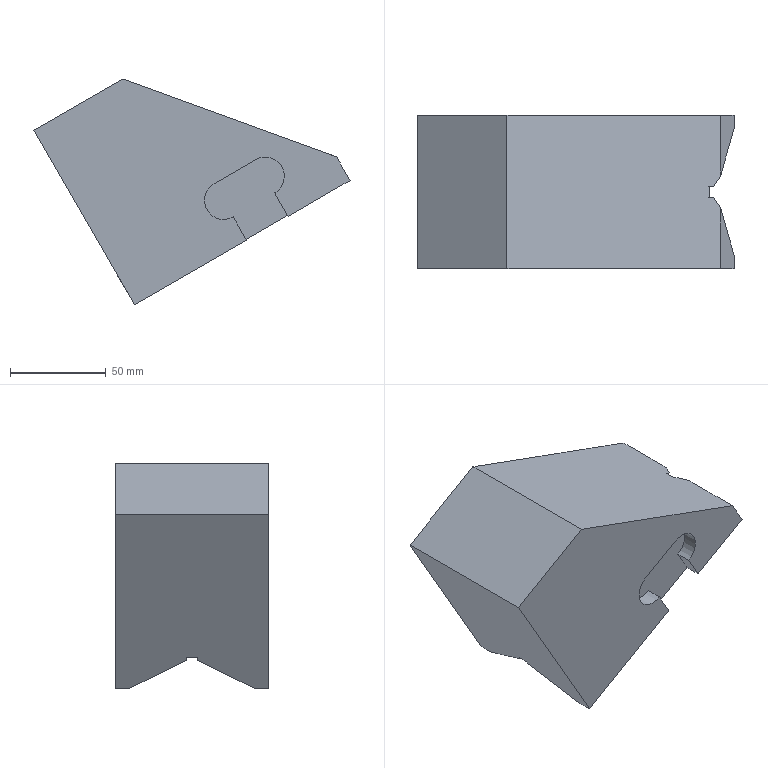Part | NX | features solid 2 | 1 solid | 28 faces | box 164.943 x 80 x 117.764 mm | volume 713626 mm3 | plane 24 | cylinder 4 | commonest cylinder face diameters 20 x4
STEP:
#1=CARTESIAN_POINT('',(760.874,-629.051,126.432));
#2=VERTEX_POINT('',#1);
#3=CARTESIAN_POINT('',(872.234,-629.052,85.9));
#4=VERTEX_POINT('',#3);
#5=CARTESIAN_POINT('',(761.219,-629.051,126.306));
#6=DIRECTION('',(0.9397,-0.000001618,-0.342));
#7=VECTOR('',#6,1000.);
#8=LINE('',#5,#7);
#9=EDGE_CURVE('',#2,#4,#8,.T.);
#10=ORIENTED_EDGE('',*,*,#9,.T.);
#11=CARTESIAN_POINT('',(879.343,-629.052,73.586));
#12=VERTEX_POINT('',#11);
#13=CARTESIAN_POINT('',(853.093,-629.052,119.052));
#14=DIRECTION('',(0.5,-0.000000963,-0.866));
#15=VECTOR('',#14,1000.);
#16=LINE('',#13,#15);
#17=EDGE_CURVE('',#4,#12,#16,.T.);
#18=ORIENTED_EDGE('',*,*,#17,.T.);
#19=CARTESIAN_POINT('',(847.008,-629.052,54.917));
#20=VERTEX_POINT('',#19);
#21=CARTESIAN_POINT('',(823.192,-629.051,41.167));
#22=DIRECTION('',(-0.866,0.00000137,-0.5));
#23=VECTOR('',#22,1000.);
#24=LINE('',#21,#23);
#25=EDGE_CURVE('',#12,#20,#24,.T.);
#26=ORIENTED_EDGE('',*,*,#25,.T.);
#27=CARTESIAN_POINT('',(840.008,-629.051,67.042));
#28=VERTEX_POINT('',#27);
#29=CARTESIAN_POINT('',(840.008,-629.051,67.042));
#30=DIRECTION('',(-0.5,0.000000963,0.866));
#31=VECTOR('',#30,1000.);
#32=LINE('',#29,#31);
#33=EDGE_CURVE('',#20,#28,#32,.T.);
#34=ORIENTED_EDGE('',*,*,#33,.T.);
#35=CARTESIAN_POINT('',(830.008,-629.051,84.362));
#36=VERTEX_POINT('',#35);
#37=CARTESIAN_POINT('',(835.008,-629.051,75.702));
#38=DIRECTION('',(0.000001668,1.,-0.000000149));
#39=DIRECTION('',(-0.9962,0.000001649,-0.08716));
#40=AXIS2_PLACEMENT_3D('',#37,#38,#39);
#41=CIRCLE('',#40,10.);
#42=EDGE_CURVE('',#36,#28,#41,.T.);
#43=ORIENTED_EDGE('',*,*,#42,.F.);
#44=CARTESIAN_POINT('',(808.357,-629.051,71.862));
#45=VERTEX_POINT('',#44);
#46=CARTESIAN_POINT('',(808.357,-629.051,71.862));
#47=DIRECTION('',(0.866,-0.00000137,0.5));
#48=VECTOR('',#47,1000.);
#49=LINE('',#46,#48);
#50=EDGE_CURVE('',#45,#36,#49,.T.);
#51=ORIENTED_EDGE('',*,*,#50,.F.);
#52=CARTESIAN_POINT('',(818.357,-629.051,54.542));
#53=VERTEX_POINT('',#52);
#54=CARTESIAN_POINT('',(813.357,-629.051,63.202));
#55=DIRECTION('',(0.000001668,1.,-0.000000149));
#56=DIRECTION('',(-0.9962,0.000001649,-0.08716));
#57=AXIS2_PLACEMENT_3D('',#54,#55,#56);
#58=CIRCLE('',#57,10.);
#59=EDGE_CURVE('',#53,#45,#58,.T.);
#60=ORIENTED_EDGE('',*,*,#59,.F.);
#61=CARTESIAN_POINT('',(825.357,-629.051,42.417));
#62=VERTEX_POINT('',#61);
#63=CARTESIAN_POINT('',(833.357,-629.051,28.561));
#64=DIRECTION('',(-0.5,0.000000963,0.866));
#65=VECTOR('',#64,1000.);
#66=LINE('',#63,#65);
#67=EDGE_CURVE('',#62,#53,#66,.T.);
#68=ORIENTED_EDGE('',*,*,#67,.F.);
#69=CARTESIAN_POINT('',(766.9,-629.051,8.667));
#70=VERTEX_POINT('',#69);
#71=CARTESIAN_POINT('',(823.192,-629.051,41.167));
#72=DIRECTION('',(-0.866,0.00000137,-0.5));
#73=VECTOR('',#72,1000.);
#74=LINE('',#71,#73);
#75=EDGE_CURVE('',#62,#70,#74,.T.);
#76=ORIENTED_EDGE('',*,*,#75,.T.);
#77=CARTESIAN_POINT('',(714.4,-629.051,99.6));
#78=VERTEX_POINT('',#77);
#79=CARTESIAN_POINT('',(740.65,-629.051,54.134));
#80=DIRECTION('',(-0.5,0.000000963,0.866));
#81=VECTOR('',#80,1000.);
#82=LINE('',#79,#81);
#83=EDGE_CURVE('',#70,#78,#82,.T.);
#84=ORIENTED_EDGE('',*,*,#83,.T.);
#85=CARTESIAN_POINT('',(770.692,-629.051,132.1));
#86=DIRECTION('',(0.866,-0.00000137,0.5));
#87=VECTOR('',#86,1000.);
#88=LINE('',#85,#87);
#89=EDGE_CURVE('',#78,#2,#88,.T.);
#90=ORIENTED_EDGE('',*,*,#89,.T.);
#91=EDGE_LOOP('',(#10,#18,#26,#34,#43,#51,#60,#68,#76,#84,#90));
#92=FACE_BOUND('',#91,.T.);
#93=CARTESIAN_POINT('',(796.942,-629.051,86.634));
#94=DIRECTION('',(0.000001668,1.,-0.000000149));
#95=DIRECTION('',(0.866,-0.00000137,0.5));
#96=AXIS2_PLACEMENT_3D('',#93,#94,#95);
#97=PLANE('',#96);
#98=ADVANCED_FACE('',(#92),#97,.T.);
#99=CARTESIAN_POINT('',(825.357,-636.143,42.417));
#100=VERTEX_POINT('',#99);
#101=CARTESIAN_POINT('',(766.9,-636.142,8.667));
#102=VERTEX_POINT('',#101);
#103=CARTESIAN_POINT('',(879.484,-636.143,73.667));
#104=DIRECTION('',(-0.866,0.00000137,-0.5));
#105=VECTOR('',#104,1000.);
#106=LINE('',#103,#105);
#107=EDGE_CURVE('',#100,#102,#106,.T.);
#108=ORIENTED_EDGE('',*,*,#107,.T.);
#109=CARTESIAN_POINT('',(766.9,-629.051,8.667));
#110=DIRECTION('',(-0.000001668,-1.,0.000000149));
#111=VECTOR('',#110,1000.);
#112=LINE('',#109,#111);
#113=EDGE_CURVE('',#70,#102,#112,.T.);
#114=ORIENTED_EDGE('',*,*,#113,.F.);
#115=ORIENTED_EDGE('',*,*,#75,.F.);
#116=CARTESIAN_POINT('',(825.357,-629.051,42.417));
#117=DIRECTION('',(0.000001668,1.,-0.000000149));
#118=VECTOR('',#117,1000.);
#119=LINE('',#116,#118);
#120=EDGE_CURVE('',#100,#62,#119,.T.);
#121=ORIENTED_EDGE('',*,*,#120,.F.);
#122=EDGE_LOOP('',(#108,#114,#115,#121));
#123=FACE_BOUND('',#122,.T.);
#124=CARTESIAN_POINT('',(823.192,-629.051,41.167));
#125=DIRECTION('',(0.5,-0.000000963,-0.866));
#126=DIRECTION('',(0.000001668,1.,-0.000000149));
#127=AXIS2_PLACEMENT_3D('',#124,#125,#126);
#128=PLANE('',#127);
#129=ADVANCED_FACE('',(#123),#128,.T.);
#130=CARTESIAN_POINT('',(872.233,-660.77,85.9));
#131=VERTEX_POINT('',#130);
#132=CARTESIAN_POINT('',(868.493,-666.052,87.261));
#133=VERTEX_POINT('',#132);
#134=CARTESIAN_POINT('',(869.088,-665.211,87.045));
#135=DIRECTION('',(-0.5656,-0.7986,0.2059));
#136=VECTOR('',#135,1000.);
#137=LINE('',#134,#136);
#138=EDGE_CURVE('',#131,#133,#137,.T.);
#139=ORIENTED_EDGE('',*,*,#138,.T.);
#140=CARTESIAN_POINT('',(758.266,-666.051,23.622));
#141=VERTEX_POINT('',#140);
#142=CARTESIAN_POINT('',(870.849,-666.052,88.622));
#143=DIRECTION('',(-0.866,0.00000137,-0.5));
#144=VECTOR('',#143,1000.);
#145=LINE('',#142,#144);
#146=EDGE_CURVE('',#133,#141,#145,.T.);
#147=ORIENTED_EDGE('',*,*,#146,.T.);
#148=CARTESIAN_POINT('',(758.266,-666.051,23.622));
#149=DIRECTION('',(0.25,0.866,-0.433));
#150=VECTOR('',#149,1000.);
#151=LINE('',#148,#150);
#152=EDGE_CURVE('',#141,#102,#151,.T.);
#153=ORIENTED_EDGE('',*,*,#152,.T.);
#154=ORIENTED_EDGE('',*,*,#107,.F.);
#155=CARTESIAN_POINT('',(825.095,-637.051,42.872));
#156=VERTEX_POINT('',#155);
#157=CARTESIAN_POINT('',(816.723,-666.051,57.372));
#158=DIRECTION('',(0.25,0.866,-0.433));
#159=VECTOR('',#158,1000.);
#160=LINE('',#157,#159);
#161=EDGE_CURVE('',#156,#100,#160,.T.);
#162=ORIENTED_EDGE('',*,*,#161,.F.);
#163=CARTESIAN_POINT('',(846.745,-637.052,55.372));
#164=VERTEX_POINT('',#163);
#165=CARTESIAN_POINT('',(879.221,-637.052,74.122));
#166=DIRECTION('',(-0.866,0.00000137,-0.5));
#167=VECTOR('',#166,1000.);
#168=LINE('',#165,#167);
#169=EDGE_CURVE('',#164,#156,#168,.T.);
#170=ORIENTED_EDGE('',*,*,#169,.F.);
#171=CARTESIAN_POINT('',(847.008,-636.143,54.917));
#172=VERTEX_POINT('',#171);
#173=CARTESIAN_POINT('',(838.374,-666.051,69.872));
#174=DIRECTION('',(0.25,0.866,-0.433));
#175=VECTOR('',#174,1000.);
#176=LINE('',#173,#175);
#177=EDGE_CURVE('',#164,#172,#176,.T.);
#178=ORIENTED_EDGE('',*,*,#177,.T.);
#179=CARTESIAN_POINT('',(879.343,-636.143,73.586));
#180=VERTEX_POINT('',#179);
#181=CARTESIAN_POINT('',(879.484,-636.143,73.667));
#182=DIRECTION('',(-0.866,0.00000137,-0.5));
#183=VECTOR('',#182,1000.);
#184=LINE('',#181,#183);
#185=EDGE_CURVE('',#180,#172,#184,.T.);
#186=ORIENTED_EDGE('',*,*,#185,.F.);
#187=CARTESIAN_POINT('',(870.709,-666.052,88.541));
#188=DIRECTION('',(0.25,0.866,-0.433));
#189=VECTOR('',#188,1000.);
#190=LINE('',#187,#189);
#191=EDGE_CURVE('',#131,#180,#190,.T.);
#192=ORIENTED_EDGE('',*,*,#191,.F.);
#193=EDGE_LOOP('',(#139,#147,#153,#154,#162,#170,#178,#186,#192));
#194=FACE_BOUND('',#193,.T.);
#195=CARTESIAN_POINT('',(870.849,-666.052,88.622));
#196=DIRECTION('',(0.433,-0.5,-0.75));
#197=DIRECTION('',(0.25,0.866,-0.433));
#198=AXIS2_PLACEMENT_3D('',#195,#196,#197);
#199=PLANE('',#198);
#200=ADVANCED_FACE('',(#194),#199,.T.);
#201=CARTESIAN_POINT('',(879.343,-701.961,73.586));
#202=VERTEX_POINT('',#201);
#203=CARTESIAN_POINT('',(847.007,-701.96,54.917));
#204=VERTEX_POINT('',#203);
#205=CARTESIAN_POINT('',(879.483,-701.961,73.667));
#206=DIRECTION('',(-0.866,0.00000137,-0.5));
#207=VECTOR('',#206,1000.);
#208=LINE('',#205,#207);
#209=EDGE_CURVE('',#202,#204,#208,.T.);
#210=ORIENTED_EDGE('',*,*,#209,.F.);
#211=CARTESIAN_POINT('',(879.343,-709.052,73.586));
#212=VERTEX_POINT('',#211);
#213=CARTESIAN_POINT('',(879.343,-629.052,73.586));
#214=DIRECTION('',(-0.000001668,-1.,0.000000149));
#215=VECTOR('',#214,1000.);
#216=LINE('',#213,#215);
#217=EDGE_CURVE('',#202,#212,#216,.T.);
#218=ORIENTED_EDGE('',*,*,#217,.T.);
#219=CARTESIAN_POINT('',(847.007,-709.052,54.917));
#220=VERTEX_POINT('',#219);
#221=CARTESIAN_POINT('',(823.192,-709.051,41.167));
#222=DIRECTION('',(0.866,-0.00000137,0.5));
#223=VECTOR('',#222,1000.);
#224=LINE('',#221,#223);
#225=EDGE_CURVE('',#220,#212,#224,.T.);
#226=ORIENTED_EDGE('',*,*,#225,.F.);
#227=CARTESIAN_POINT('',(847.008,-629.052,54.917));
#228=DIRECTION('',(-0.000001668,-1.,0.000000149));
#229=VECTOR('',#228,1000.);
#230=LINE('',#227,#229);
#231=EDGE_CURVE('',#204,#220,#230,.T.);
#232=ORIENTED_EDGE('',*,*,#231,.F.);
#233=EDGE_LOOP('',(#210,#218,#226,#232));
#234=FACE_BOUND('',#233,.T.);
#235=CARTESIAN_POINT('',(823.192,-629.051,41.167));
#236=DIRECTION('',(0.5,-0.000000963,-0.866));
#237=DIRECTION('',(0.000001668,1.,-0.000000149));
#238=AXIS2_PLACEMENT_3D('',#235,#236,#237);
#239=PLANE('',#238);
#240=ADVANCED_FACE('',(#234),#239,.T.);
#241=CARTESIAN_POINT('',(847.008,-629.052,54.917));
#242=DIRECTION('',(0.000001668,1.,-0.000000149));
#243=VECTOR('',#242,1000.);
#244=LINE('',#241,#243);
#245=EDGE_CURVE('',#172,#20,#244,.T.);
#246=ORIENTED_EDGE('',*,*,#245,.T.);
#247=ORIENTED_EDGE('',*,*,#25,.F.);
#248=CARTESIAN_POINT('',(879.343,-629.052,73.586));
#249=DIRECTION('',(-0.000001668,-1.,0.000000149));
#250=VECTOR('',#249,1000.);
#251=LINE('',#248,#250);
#252=EDGE_CURVE('',#12,#180,#251,.T.);
#253=ORIENTED_EDGE('',*,*,#252,.T.);
#254=ORIENTED_EDGE('',*,*,#185,.T.);
#255=EDGE_LOOP('',(#246,#247,#253,#254));
#256=FACE_BOUND('',#255,.T.);
#257=CARTESIAN_POINT('',(823.192,-629.051,41.167));
#258=DIRECTION('',(0.5,-0.000000963,-0.866));
#259=DIRECTION('',(0.000001668,1.,-0.000000149));
#260=AXIS2_PLACEMENT_3D('',#257,#258,#259);
#261=PLANE('',#260);
#262=ADVANCED_FACE('',(#256),#261,.T.);
#263=CARTESIAN_POINT('',(825.357,-701.96,42.417));
#264=VERTEX_POINT('',#263);
#265=CARTESIAN_POINT('',(825.357,-709.051,42.417));
#266=VERTEX_POINT('',#265);
#267=CARTESIAN_POINT('',(825.357,-629.051,42.417));
#268=DIRECTION('',(-0.000001668,-1.,0.000000149));
#269=VECTOR('',#268,1000.);
#270=LINE('',#267,#269);
#271=EDGE_CURVE('',#264,#266,#270,.T.);
#272=ORIENTED_EDGE('',*,*,#271,.T.);
#273=CARTESIAN_POINT('',(766.9,-709.051,8.667));
#274=VERTEX_POINT('',#273);
#275=CARTESIAN_POINT('',(823.192,-709.051,41.167));
#276=DIRECTION('',(0.866,-0.00000137,0.5));
#277=VECTOR('',#276,1000.);
#278=LINE('',#275,#277);
#279=EDGE_CURVE('',#274,#266,#278,.T.);
#280=ORIENTED_EDGE('',*,*,#279,.F.);
#281=CARTESIAN_POINT('',(766.9,-701.96,8.667));
#282=VERTEX_POINT('',#281);
#283=CARTESIAN_POINT('',(766.9,-629.051,8.667));
#284=DIRECTION('',(-0.000001668,-1.,0.000000149));
#285=VECTOR('',#284,1000.);
#286=LINE('',#283,#285);
#287=EDGE_CURVE('',#282,#274,#286,.T.);
#288=ORIENTED_EDGE('',*,*,#287,.F.);
#289=CARTESIAN_POINT('',(879.483,-701.961,73.667));
#290=DIRECTION('',(-0.866,0.00000137,-0.5));
#291=VECTOR('',#290,1000.);
#292=LINE('',#289,#291);
#293=EDGE_CURVE('',#264,#282,#292,.T.);
#294=ORIENTED_EDGE('',*,*,#293,.F.);
#295=EDGE_LOOP('',(#272,#280,#288,#294));
#296=FACE_BOUND('',#295,.T.);
#297=CARTESIAN_POINT('',(823.192,-629.051,41.167));
#298=DIRECTION('',(0.5,-0.000000963,-0.866));
#299=DIRECTION('',(0.000001668,1.,-0.000000149));
#300=AXIS2_PLACEMENT_3D('',#297,#298,#299);
#301=PLANE('',#300);
#302=ADVANCED_FACE('',(#296),#301,.T.);
#303=CARTESIAN_POINT('',(872.233,-709.052,85.9));
#304=DIRECTION('',(0.000001668,1.,-0.000000149));
#305=VECTOR('',#304,1000.);
#306=LINE('',#303,#305);
#307=EDGE_CURVE('',#131,#4,#306,.T.);
#308=ORIENTED_EDGE('',*,*,#307,.F.);
#309=ORIENTED_EDGE('',*,*,#191,.T.);
#310=ORIENTED_EDGE('',*,*,#252,.F.);
#311=ORIENTED_EDGE('',*,*,#17,.F.);
#312=EDGE_LOOP('',(#308,#309,#310,#311));
#313=FACE_BOUND('',#312,.T.);
#314=CARTESIAN_POINT('',(853.093,-629.052,119.052));
#315=DIRECTION('',(0.866,-0.00000137,0.5));
#316=DIRECTION('',(-0.000001668,-1.,0.000000149));
#317=AXIS2_PLACEMENT_3D('',#314,#315,#316);
#318=PLANE('',#317);
#319=ADVANCED_FACE('',(#313),#318,.T.);
#320=CARTESIAN_POINT('',(872.233,-709.052,85.9));
#321=VERTEX_POINT('',#320);
#322=CARTESIAN_POINT('',(872.233,-677.333,85.9));
#323=VERTEX_POINT('',#322);
#324=CARTESIAN_POINT('',(872.233,-709.052,85.9));
#325=DIRECTION('',(0.000001668,1.,-0.000000149));
#326=VECTOR('',#325,1000.);
#327=LINE('',#324,#326);
#328=EDGE_CURVE('',#321,#323,#327,.T.);
#329=ORIENTED_EDGE('',*,*,#328,.F.);
#330=CARTESIAN_POINT('',(853.093,-709.052,119.052));
#331=DIRECTION('',(-0.5,0.000000963,0.866));
#332=VECTOR('',#331,1000.);
#333=LINE('',#330,#332);
#334=EDGE_CURVE('',#212,#321,#333,.T.);
#335=ORIENTED_EDGE('',*,*,#334,.F.);
#336=ORIENTED_EDGE('',*,*,#217,.F.);
#337=CARTESIAN_POINT('',(879.343,-701.961,73.586));
#338=DIRECTION('',(-0.25,0.866,0.433));
#339=VECTOR('',#338,1000.);
#340=LINE('',#337,#339);
#341=EDGE_CURVE('',#202,#323,#340,.T.);
#342=ORIENTED_EDGE('',*,*,#341,.T.);
#343=EDGE_LOOP('',(#329,#335,#336,#342));
#344=FACE_BOUND('',#343,.T.);
#345=CARTESIAN_POINT('',(853.093,-629.052,119.052));
#346=DIRECTION('',(0.866,-0.00000137,0.5));
#347=DIRECTION('',(-0.000001668,-1.,0.000000149));
#348=AXIS2_PLACEMENT_3D('',#345,#346,#347);
#349=PLANE('',#348);
#350=ADVANCED_FACE('',(#344),#349,.T.);
#351=CARTESIAN_POINT('',(757.4,-666.051,25.122));
#352=VERTEX_POINT('',#351);
#353=CARTESIAN_POINT('',(757.4,-666.051,25.122));
#354=DIRECTION('',(0.5,-0.000000963,-0.866));
#355=VECTOR('',#354,1000.);
#356=LINE('',#353,#355);
#357=EDGE_CURVE('',#352,#141,#356,.T.);
#358=ORIENTED_EDGE('',*,*,#357,.F.);
#359=CARTESIAN_POINT('',(757.4,-672.051,25.122));
#360=VERTEX_POINT('',#359);
#361=CARTESIAN_POINT('',(757.4,-672.051,25.122));
#362=DIRECTION('',(0.000001668,1.,-0.000000149));
#363=VECTOR('',#362,1000.);
#364=LINE('',#361,#363);
#365=EDGE_CURVE('',#360,#352,#364,.T.);
#366=ORIENTED_EDGE('',*,*,#365,.F.);
#367=CARTESIAN_POINT('',(758.266,-672.051,23.622));
#368=VERTEX_POINT('',#367);
#369=CARTESIAN_POINT('',(758.266,-672.051,23.622));
#370=DIRECTION('',(-0.5,0.000000963,0.866));
#371=VECTOR('',#370,1000.);
#372=LINE('',#369,#371);
#373=EDGE_CURVE('',#368,#360,#372,.T.);
#374=ORIENTED_EDGE('',*,*,#373,.F.);
#375=CARTESIAN_POINT('',(766.9,-701.96,8.667));
#376=DIRECTION('',(-0.25,0.866,0.433));
#377=VECTOR('',#376,1000.);
#378=LINE('',#375,#377);
#379=EDGE_CURVE('',#282,#368,#378,.T.);
#380=ORIENTED_EDGE('',*,*,#379,.F.);
#381=ORIENTED_EDGE('',*,*,#287,.T.);
#382=CARTESIAN_POINT('',(714.4,-709.051,99.6));
#383=VERTEX_POINT('',#382);
#384=CARTESIAN_POINT('',(740.65,-709.051,54.134));
#385=DIRECTION('',(0.5,-0.000000963,-0.866));
#386=VECTOR('',#385,1000.);
#387=LINE('',#384,#386);
#388=EDGE_CURVE('',#383,#274,#387,.T.);
#389=ORIENTED_EDGE('',*,*,#388,.F.);
#390=CARTESIAN_POINT('',(714.4,-629.051,99.6));
#391=DIRECTION('',(-0.000001668,-1.,0.000000149));
#392=VECTOR('',#391,1000.);
#393=LINE('',#390,#392);
#394=EDGE_CURVE('',#78,#383,#393,.T.);
#395=ORIENTED_EDGE('',*,*,#394,.F.);
#396=ORIENTED_EDGE('',*,*,#83,.F.);
#397=ORIENTED_EDGE('',*,*,#113,.T.);
#398=ORIENTED_EDGE('',*,*,#152,.F.);
#399=EDGE_LOOP('',(#358,#366,#374,#380,#381,#389,#395,#396,#397,#398));
#400=FACE_BOUND('',#399,.T.);
#401=CARTESIAN_POINT('',(740.65,-629.051,54.134));
#402=DIRECTION('',(-0.866,0.00000137,-0.5));
#403=DIRECTION('',(0.000001668,1.,-0.000000149));
#404=AXIS2_PLACEMENT_3D('',#401,#402,#403);
#405=PLANE('',#404);
#406=ADVANCED_FACE('',(#400),#405,.T.);
#407=CARTESIAN_POINT('',(760.874,-709.051,126.432));
#408=VERTEX_POINT('',#407);
#409=CARTESIAN_POINT('',(761.219,-709.051,126.306));
#410=DIRECTION('',(0.9397,-0.000001618,-0.342));
#411=VECTOR('',#410,1000.);
#412=LINE('',#409,#411);
#413=EDGE_CURVE('',#408,#321,#412,.T.);
#414=ORIENTED_EDGE('',*,*,#413,.F.);
#415=CARTESIAN_POINT('',(770.692,-709.051,132.1));
#416=DIRECTION('',(-0.866,0.00000137,-0.5));
#417=VECTOR('',#416,1000.);
#418=LINE('',#415,#417);
#419=EDGE_CURVE('',#408,#383,#418,.T.);
#420=ORIENTED_EDGE('',*,*,#419,.T.);
#421=ORIENTED_EDGE('',*,*,#388,.T.);
#422=ORIENTED_EDGE('',*,*,#279,.T.);
#423=CARTESIAN_POINT('',(818.357,-709.051,54.542));
#424=VERTEX_POINT('',#423);
#425=CARTESIAN_POINT('',(833.357,-709.051,28.561));
#426=DIRECTION('',(-0.5,0.000000963,0.866));
#427=VECTOR('',#426,1000.);
#428=LINE('',#425,#427);
#429=EDGE_CURVE('',#266,#424,#428,.T.);
#430=ORIENTED_EDGE('',*,*,#429,.T.);
#431=CARTESIAN_POINT('',(808.357,-709.051,71.862));
#432=VERTEX_POINT('',#431);
#433=CARTESIAN_POINT('',(813.357,-709.051,63.202));
#434=DIRECTION('',(0.000001668,1.,-0.000000149));
#435=DIRECTION('',(-0.9962,0.000001649,-0.08716));
#436=AXIS2_PLACEMENT_3D('',#433,#434,#435);
#437=CIRCLE('',#436,10.);
#438=EDGE_CURVE('',#424,#432,#437,.T.);
#439=ORIENTED_EDGE('',*,*,#438,.T.);
#440=CARTESIAN_POINT('',(830.007,-709.051,84.362));
#441=VERTEX_POINT('',#440);
#442=CARTESIAN_POINT('',(830.007,-709.051,84.362));
#443=DIRECTION('',(-0.866,0.00000137,-0.5));
#444=VECTOR('',#443,1000.);
#445=LINE('',#442,#444);
#446=EDGE_CURVE('',#441,#432,#445,.T.);
#447=ORIENTED_EDGE('',*,*,#446,.F.);
#448=CARTESIAN_POINT('',(840.007,-709.051,67.042));
#449=VERTEX_POINT('',#448);
#450=CARTESIAN_POINT('',(835.007,-709.051,75.702));
#451=DIRECTION('',(0.000001668,1.,-0.000000149));
#452=DIRECTION('',(-0.9962,0.000001649,-0.08716));
#453=AXIS2_PLACEMENT_3D('',#450,#451,#452);
#454=CIRCLE('',#453,10.);
#455=EDGE_CURVE('',#441,#449,#454,.T.);
#456=ORIENTED_EDGE('',*,*,#455,.T.);
#457=CARTESIAN_POINT('',(855.007,-709.052,41.061));
#458=DIRECTION('',(-0.5,0.000000963,0.866));
#459=VECTOR('',#458,1000.);
#460=LINE('',#457,#459);
#461=EDGE_CURVE('',#220,#449,#460,.T.);
#462=ORIENTED_EDGE('',*,*,#461,.F.);
#463=ORIENTED_EDGE('',*,*,#225,.T.);
#464=ORIENTED_EDGE('',*,*,#334,.T.);
#465=EDGE_LOOP('',(#414,#420,#421,#422,#430,#439,#447,#456,#462,#463,#464));
#466=FACE_BOUND('',#465,.T.);
#467=CARTESIAN_POINT('',(796.942,-709.051,86.634));
#468=DIRECTION('',(-0.000001668,-1.,0.000000149));
#469=DIRECTION('',(-0.866,0.00000137,-0.5));
#470=AXIS2_PLACEMENT_3D('',#467,#468,#469);
#471=PLANE('',#470);
#472=ADVANCED_FACE('',(#466),#471,.T.);
#473=CARTESIAN_POINT('',(760.874,-629.051,126.432));
#474=DIRECTION('',(0.000001668,1.,-0.000000149));
#475=VECTOR('',#474,1000.);
#476=LINE('',#473,#475);
#477=EDGE_CURVE('',#408,#2,#476,.T.);
#478=ORIENTED_EDGE('',*,*,#477,.T.);
#479=ORIENTED_EDGE('',*,*,#89,.F.);
#480=ORIENTED_EDGE('',*,*,#394,.T.);
#481=ORIENTED_EDGE('',*,*,#419,.F.);
#482=EDGE_LOOP('',(#478,#479,#480,#481));
#483=FACE_BOUND('',#482,.T.);
#484=CARTESIAN_POINT('',(770.692,-629.051,132.1));
#485=DIRECTION('',(-0.5,0.000000963,0.866));
#486=DIRECTION('',(-0.000001668,-1.,0.000000149));
#487=AXIS2_PLACEMENT_3D('',#484,#485,#486);
#488=PLANE('',#487);
#489=ADVANCED_FACE('',(#483),#488,.T.);
#490=CARTESIAN_POINT('',(866.368,-672.052,88.035));
#491=VERTEX_POINT('',#490);
#492=CARTESIAN_POINT('',(868.493,-672.052,87.261));
#493=VERTEX_POINT('',#492);
#494=CARTESIAN_POINT('',(870.137,-672.052,86.663));
#495=DIRECTION('',(0.9397,-0.000001618,-0.342));
#496=VECTOR('',#495,1000.);
#497=LINE('',#494,#496);
#498=EDGE_CURVE('',#491,#493,#497,.T.);
#499=ORIENTED_EDGE('',*,*,#498,.T.);
#500=CARTESIAN_POINT('',(870.849,-672.052,88.622));
#501=DIRECTION('',(-0.866,0.00000137,-0.5));
#502=VECTOR('',#501,1000.);
#503=LINE('',#500,#502);
#504=EDGE_CURVE('',#493,#368,#503,.T.);
#505=ORIENTED_EDGE('',*,*,#504,.T.);
#506=ORIENTED_EDGE('',*,*,#373,.T.);
#507=CARTESIAN_POINT('',(869.983,-672.052,90.122));
#508=DIRECTION('',(-0.866,0.00000137,-0.5));
#509=VECTOR('',#508,1000.);
#510=LINE('',#507,#509);
#511=EDGE_CURVE('',#491,#360,#510,.T.);
#512=ORIENTED_EDGE('',*,*,#511,.F.);
#513=EDGE_LOOP('',(#499,#505,#506,#512));
#514=FACE_BOUND('',#513,.T.);
#515=CARTESIAN_POINT('',(870.849,-672.052,88.622));
#516=DIRECTION('',(0.000001668,1.,-0.000000149));
#517=DIRECTION('',(-0.5,0.000000963,0.866));
#518=AXIS2_PLACEMENT_3D('',#515,#516,#517);
#519=PLANE('',#518);
#520=ADVANCED_FACE('',(#514),#519,.T.);
#521=CARTESIAN_POINT('',(866.368,-666.052,88.035));
#522=VERTEX_POINT('',#521);
#523=CARTESIAN_POINT('',(866.368,-672.052,88.035));
#524=DIRECTION('',(-0.000001668,-1.,0.000000149));
#525=VECTOR('',#524,1000.);
#526=LINE('',#523,#525);
#527=EDGE_CURVE('',#522,#491,#526,.T.);
#528=ORIENTED_EDGE('',*,*,#527,.T.);
#529=ORIENTED_EDGE('',*,*,#511,.T.);
#530=ORIENTED_EDGE('',*,*,#365,.T.);
#531=CARTESIAN_POINT('',(869.983,-666.052,90.122));
#532=DIRECTION('',(-0.866,0.00000137,-0.5));
#533=VECTOR('',#532,1000.);
#534=LINE('',#531,#533);
#535=EDGE_CURVE('',#522,#352,#534,.T.);
#536=ORIENTED_EDGE('',*,*,#535,.F.);
#537=EDGE_LOOP('',(#528,#529,#530,#536));
#538=FACE_BOUND('',#537,.T.);
#539=CARTESIAN_POINT('',(869.983,-672.052,90.122));
#540=DIRECTION('',(0.5,-0.000000963,-0.866));
#541=DIRECTION('',(0.000001668,1.,-0.000000149));
#542=AXIS2_PLACEMENT_3D('',#539,#540,#541);
#543=PLANE('',#542);
#544=ADVANCED_FACE('',(#538),#543,.T.);
#545=CARTESIAN_POINT('',(868.89,-666.052,87.117));
#546=DIRECTION('',(-0.9397,0.000001618,0.342));
#547=VECTOR('',#546,1000.);
#548=LINE('',#545,#547);
#549=EDGE_CURVE('',#133,#522,#548,.T.);
#550=ORIENTED_EDGE('',*,*,#549,.T.);
#551=ORIENTED_EDGE('',*,*,#535,.T.);
#552=ORIENTED_EDGE('',*,*,#357,.T.);
#553=ORIENTED_EDGE('',*,*,#146,.F.);
#554=EDGE_LOOP('',(#550,#551,#552,#553));
#555=FACE_BOUND('',#554,.T.);
#556=CARTESIAN_POINT('',(869.983,-666.052,90.122));
#557=DIRECTION('',(-0.000001668,-1.,0.000000149));
#558=DIRECTION('',(0.5,-0.000000963,-0.866));
#559=AXIS2_PLACEMENT_3D('',#556,#557,#558);
#560=PLANE('',#559);
#561=ADVANCED_FACE('',(#555),#560,.T.);
#562=CARTESIAN_POINT('',(887.1,-698.325,80.489));
#563=DIRECTION('',(0.5656,-0.7986,-0.2059));
#564=VECTOR('',#563,1000.);
#565=LINE('',#562,#564);
#566=EDGE_CURVE('',#493,#323,#565,.T.);
#567=ORIENTED_EDGE('',*,*,#566,.T.);
#568=ORIENTED_EDGE('',*,*,#341,.F.);
#569=ORIENTED_EDGE('',*,*,#209,.T.);
#570=CARTESIAN_POINT('',(846.745,-701.052,55.372));
#571=VERTEX_POINT('',#570);
#572=CARTESIAN_POINT('',(847.007,-701.96,54.917));
#573=DIRECTION('',(0.25,-0.866,-0.433));
#574=VECTOR('',#573,1000.);
#575=LINE('',#572,#574);
#576=EDGE_CURVE('',#571,#204,#575,.T.);
#577=ORIENTED_EDGE('',*,*,#576,.F.);
#578=CARTESIAN_POINT('',(825.094,-701.051,42.872));
#579=VERTEX_POINT('',#578);
#580=CARTESIAN_POINT('',(879.221,-701.052,74.122));
#581=DIRECTION('',(0.866,-0.00000137,0.5));
#582=VECTOR('',#581,1000.);
#583=LINE('',#580,#582);
#584=EDGE_CURVE('',#579,#571,#583,.T.);
#585=ORIENTED_EDGE('',*,*,#584,.F.);
#586=CARTESIAN_POINT('',(825.357,-701.96,42.417));
#587=DIRECTION('',(0.25,-0.866,-0.433));
#588=VECTOR('',#587,1000.);
#589=LINE('',#586,#588);
#590=EDGE_CURVE('',#579,#264,#589,.T.);
#591=ORIENTED_EDGE('',*,*,#590,.T.);
#592=ORIENTED_EDGE('',*,*,#293,.T.);
#593=ORIENTED_EDGE('',*,*,#379,.T.);
#594=ORIENTED_EDGE('',*,*,#504,.F.);
#595=EDGE_LOOP('',(#567,#568,#569,#577,#585,#591,#592,#593,#594));
#596=FACE_BOUND('',#595,.T.);
#597=CARTESIAN_POINT('',(879.483,-701.961,73.667));
#598=DIRECTION('',(0.433,0.5,-0.75));
#599=DIRECTION('',(-0.25,0.866,0.433));
#600=AXIS2_PLACEMENT_3D('',#597,#598,#599);
#601=PLANE('',#600);
#602=ADVANCED_FACE('',(#596),#601,.T.);
#603=ORIENTED_EDGE('',*,*,#438,.F.);
#604=CARTESIAN_POINT('',(818.357,-701.051,54.542));
#605=VERTEX_POINT('',#604);
#606=CARTESIAN_POINT('',(818.357,-701.051,54.542));
#607=DIRECTION('',(-0.000001668,-1.,0.000000149));
#608=VECTOR('',#607,1000.);
#609=LINE('',#606,#608);
#610=EDGE_CURVE('',#605,#424,#609,.T.);
#611=ORIENTED_EDGE('',*,*,#610,.F.);
#612=CARTESIAN_POINT('',(808.357,-701.051,71.862));
#613=VERTEX_POINT('',#612);
#614=CARTESIAN_POINT('',(813.357,-701.051,63.202));
#615=DIRECTION('',(0.000001668,1.,-0.000000149));
#616=DIRECTION('',(-0.9962,0.000001649,-0.08716));
#617=AXIS2_PLACEMENT_3D('',#614,#615,#616);
#618=CIRCLE('',#617,10.);
#619=EDGE_CURVE('',#605,#613,#618,.T.);
#620=ORIENTED_EDGE('',*,*,#619,.T.);
#621=CARTESIAN_POINT('',(808.357,-701.051,71.862));
#622=DIRECTION('',(-0.000001668,-1.,0.000000149));
#623=VECTOR('',#622,1000.);
#624=LINE('',#621,#623);
#625=EDGE_CURVE('',#613,#432,#624,.T.);
#626=ORIENTED_EDGE('',*,*,#625,.T.);
#627=EDGE_LOOP('',(#603,#611,#620,#626));
#628=FACE_BOUND('',#627,.T.);
#629=CARTESIAN_POINT('',(813.357,-701.051,63.202));
#630=DIRECTION('',(-0.000001668,-1.,0.000000149));
#631=DIRECTION('',(-1.,0.000001668,0.000000502));
#632=AXIS2_PLACEMENT_3D('',#629,#630,#631);
#633=CYLINDRICAL_SURFACE('',#632,10.);
#634=ADVANCED_FACE('',(#628),#633,.F.);
#635=ORIENTED_EDGE('',*,*,#446,.T.);
#636=ORIENTED_EDGE('',*,*,#625,.F.);
#637=CARTESIAN_POINT('',(830.007,-701.051,84.362));
#638=VERTEX_POINT('',#637);
#639=CARTESIAN_POINT('',(830.007,-701.051,84.362));
#640=DIRECTION('',(-0.866,0.00000137,-0.5));
#641=VECTOR('',#640,1000.);
#642=LINE('',#639,#641);
#643=EDGE_CURVE('',#638,#613,#642,.T.);
#644=ORIENTED_EDGE('',*,*,#643,.F.);
#645=CARTESIAN_POINT('',(830.007,-701.051,84.362));
#646=DIRECTION('',(-0.000001668,-1.,0.000000149));
#647=VECTOR('',#646,1000.);
#648=LINE('',#645,#647);
#649=EDGE_CURVE('',#638,#441,#648,.T.);
#650=ORIENTED_EDGE('',*,*,#649,.T.);
#651=EDGE_LOOP('',(#635,#636,#644,#650));
#652=FACE_BOUND('',#651,.T.);
#653=CARTESIAN_POINT('',(830.007,-701.051,84.362));
#654=DIRECTION('',(0.5,-0.000000963,-0.866));
#655=DIRECTION('',(-0.866,0.00000137,-0.5));
#656=AXIS2_PLACEMENT_3D('',#653,#654,#655);
#657=PLANE('',#656);
#658=ADVANCED_FACE('',(#652),#657,.T.);
#659=ORIENTED_EDGE('',*,*,#455,.F.);
#660=ORIENTED_EDGE('',*,*,#649,.F.);
#661=CARTESIAN_POINT('',(840.007,-701.051,67.042));
#662=VERTEX_POINT('',#661);
#663=CARTESIAN_POINT('',(835.007,-701.051,75.702));
#664=DIRECTION('',(0.000001668,1.,-0.000000149));
#665=DIRECTION('',(-0.9962,0.000001649,-0.08716));
#666=AXIS2_PLACEMENT_3D('',#663,#664,#665);
#667=CIRCLE('',#666,10.);
#668=EDGE_CURVE('',#638,#662,#667,.T.);
#669=ORIENTED_EDGE('',*,*,#668,.T.);
#670=CARTESIAN_POINT('',(840.007,-701.051,67.042));
#671=DIRECTION('',(-0.000001668,-1.,0.000000149));
#672=VECTOR('',#671,1000.);
#673=LINE('',#670,#672);
#674=EDGE_CURVE('',#662,#449,#673,.T.);
#675=ORIENTED_EDGE('',*,*,#674,.T.);
#676=EDGE_LOOP('',(#659,#660,#669,#675));
#677=FACE_BOUND('',#676,.T.);
#678=CARTESIAN_POINT('',(835.007,-701.051,75.702));
#679=DIRECTION('',(-0.000001668,-1.,0.000000149));
#680=DIRECTION('',(-1.,0.000001668,0.000000502));
#681=AXIS2_PLACEMENT_3D('',#678,#679,#680);
#682=CYLINDRICAL_SURFACE('',#681,10.);
#683=ADVANCED_FACE('',(#677),#682,.F.);
#684=ORIENTED_EDGE('',*,*,#668,.F.);
#685=ORIENTED_EDGE('',*,*,#643,.T.);
#686=ORIENTED_EDGE('',*,*,#619,.F.);
#687=CARTESIAN_POINT('',(833.357,-701.051,28.561));
#688=DIRECTION('',(-0.5,0.000000963,0.866));
#689=VECTOR('',#688,1000.);
#690=LINE('',#687,#689);
#691=EDGE_CURVE('',#579,#605,#690,.T.);
#692=ORIENTED_EDGE('',*,*,#691,.F.);
#693=ORIENTED_EDGE('',*,*,#584,.T.);
#694=CARTESIAN_POINT('',(855.007,-701.052,41.061));
#695=DIRECTION('',(-0.5,0.000000963,0.866));
#696=VECTOR('',#695,1000.);
#697=LINE('',#694,#696);
#698=EDGE_CURVE('',#571,#662,#697,.T.);
#699=ORIENTED_EDGE('',*,*,#698,.T.);
#700=EDGE_LOOP('',(#684,#685,#686,#692,#693,#699));
#701=FACE_BOUND('',#700,.T.);
#702=CARTESIAN_POINT('',(813.357,-701.051,63.202));
#703=DIRECTION('',(-0.000001668,-1.,0.000000149));
#704=DIRECTION('',(-1.,0.000001668,0.000000502));
#705=AXIS2_PLACEMENT_3D('',#702,#703,#704);
#706=PLANE('',#705);
#707=ADVANCED_FACE('',(#701),#706,.T.);
#708=ORIENTED_EDGE('',*,*,#271,.F.);
#709=ORIENTED_EDGE('',*,*,#590,.F.);
#710=ORIENTED_EDGE('',*,*,#691,.T.);
#711=ORIENTED_EDGE('',*,*,#610,.T.);
#712=ORIENTED_EDGE('',*,*,#429,.F.);
#713=EDGE_LOOP('',(#708,#709,#710,#711,#712));
#714=FACE_BOUND('',#713,.T.);
#715=CARTESIAN_POINT('',(833.357,-701.051,28.561));
#716=DIRECTION('',(-0.866,0.00000137,-0.5));
#717=DIRECTION('',(-0.5,0.000000963,0.866));
#718=AXIS2_PLACEMENT_3D('',#715,#716,#717);
#719=PLANE('',#718);
#720=ADVANCED_FACE('',(#714),#719,.F.);
#721=ORIENTED_EDGE('',*,*,#576,.T.);
#722=ORIENTED_EDGE('',*,*,#231,.T.);
#723=ORIENTED_EDGE('',*,*,#461,.T.);
#724=ORIENTED_EDGE('',*,*,#674,.F.);
#725=ORIENTED_EDGE('',*,*,#698,.F.);
#726=EDGE_LOOP('',(#721,#722,#723,#724,#725));
#727=FACE_BOUND('',#726,.T.);
#728=CARTESIAN_POINT('',(855.007,-701.052,41.061));
#729=DIRECTION('',(-0.866,0.00000137,-0.5));
#730=DIRECTION('',(-0.5,0.000000963,0.866));
#731=AXIS2_PLACEMENT_3D('',#728,#729,#730);
#732=PLANE('',#731);
#733=ADVANCED_FACE('',(#727),#732,.T.);
#734=ORIENTED_EDGE('',*,*,#50,.T.);
#735=CARTESIAN_POINT('',(830.008,-637.051,84.362));
#736=VERTEX_POINT('',#735);
#737=CARTESIAN_POINT('',(830.008,-629.051,84.362));
#738=DIRECTION('',(-0.000001668,-1.,0.000000149));
#739=VECTOR('',#738,1000.);
#740=LINE('',#737,#739);
#741=EDGE_CURVE('',#36,#736,#740,.T.);
#742=ORIENTED_EDGE('',*,*,#741,.T.);
#743=CARTESIAN_POINT('',(808.357,-637.051,71.862));
#744=VERTEX_POINT('',#743);
#745=CARTESIAN_POINT('',(808.357,-637.051,71.862));
#746=DIRECTION('',(0.866,-0.00000137,0.5));
#747=VECTOR('',#746,1000.);
#748=LINE('',#745,#747);
#749=EDGE_CURVE('',#744,#736,#748,.T.);
#750=ORIENTED_EDGE('',*,*,#749,.F.);
#751=CARTESIAN_POINT('',(808.357,-637.051,71.862));
#752=DIRECTION('',(0.000001668,1.,-0.000000149));
#753=VECTOR('',#752,1000.);
#754=LINE('',#751,#753);
#755=EDGE_CURVE('',#744,#45,#754,.T.);
#756=ORIENTED_EDGE('',*,*,#755,.T.);
#757=EDGE_LOOP('',(#734,#742,#750,#756));
#758=FACE_BOUND('',#757,.T.);
#759=CARTESIAN_POINT('',(808.357,-637.051,71.862));
#760=DIRECTION('',(0.5,-0.000000963,-0.866));
#761=DIRECTION('',(-0.866,0.00000137,-0.5));
#762=AXIS2_PLACEMENT_3D('',#759,#760,#761);
#763=PLANE('',#762);
#764=ADVANCED_FACE('',(#758),#763,.T.);
#765=CARTESIAN_POINT('',(818.357,-637.051,54.542));
#766=VERTEX_POINT('',#765);
#767=CARTESIAN_POINT('',(818.357,-629.051,54.542));
#768=DIRECTION('',(-0.000001668,-1.,0.000000149));
#769=VECTOR('',#768,1000.);
#770=LINE('',#767,#769);
#771=EDGE_CURVE('',#53,#766,#770,.T.);
#772=ORIENTED_EDGE('',*,*,#771,.T.);
#773=CARTESIAN_POINT('',(833.357,-637.051,28.561));
#774=DIRECTION('',(-0.5,0.000000963,0.866));
#775=VECTOR('',#774,1000.);
#776=LINE('',#773,#775);
#777=EDGE_CURVE('',#156,#766,#776,.T.);
#778=ORIENTED_EDGE('',*,*,#777,.F.);
#779=ORIENTED_EDGE('',*,*,#161,.T.);
#780=ORIENTED_EDGE('',*,*,#120,.T.);
#781=ORIENTED_EDGE('',*,*,#67,.T.);
#782=EDGE_LOOP('',(#772,#778,#779,#780,#781));
#783=FACE_BOUND('',#782,.T.);
#784=CARTESIAN_POINT('',(833.357,-637.051,28.561));
#785=DIRECTION('',(0.866,-0.00000137,0.5));
#786=DIRECTION('',(0.5,-0.000000963,-0.866));
#787=AXIS2_PLACEMENT_3D('',#784,#785,#786);
#788=PLANE('',#787);
#789=ADVANCED_FACE('',(#783),#788,.T.);
#790=ORIENTED_EDGE('',*,*,#33,.F.);
#791=ORIENTED_EDGE('',*,*,#245,.F.);
#792=ORIENTED_EDGE('',*,*,#177,.F.);
#793=CARTESIAN_POINT('',(840.008,-637.051,67.042));
#794=VERTEX_POINT('',#793);
#795=CARTESIAN_POINT('',(840.008,-637.051,67.042));
#796=DIRECTION('',(-0.5,0.000000963,0.866));
#797=VECTOR('',#796,1000.);
#798=LINE('',#795,#797);
#799=EDGE_CURVE('',#164,#794,#798,.T.);
#800=ORIENTED_EDGE('',*,*,#799,.T.);
#801=CARTESIAN_POINT('',(840.008,-629.051,67.042));
#802=DIRECTION('',(-0.000001668,-1.,0.000000149));
#803=VECTOR('',#802,1000.);
#804=LINE('',#801,#803);
#805=EDGE_CURVE('',#28,#794,#804,.T.);
#806=ORIENTED_EDGE('',*,*,#805,.F.);
#807=EDGE_LOOP('',(#790,#791,#792,#800,#806));
#808=FACE_BOUND('',#807,.T.);
#809=CARTESIAN_POINT('',(840.008,-637.051,67.042));
#810=DIRECTION('',(0.866,-0.00000137,0.5));
#811=DIRECTION('',(0.5,-0.000000963,-0.866));
#812=AXIS2_PLACEMENT_3D('',#809,#810,#811);
#813=PLANE('',#812);
#814=ADVANCED_FACE('',(#808),#813,.F.);
#815=CARTESIAN_POINT('',(835.008,-637.051,75.702));
#816=DIRECTION('',(0.000001668,1.,-0.000000149));
#817=DIRECTION('',(-0.9962,0.000001649,-0.08716));
#818=AXIS2_PLACEMENT_3D('',#815,#816,#817);
#819=CIRCLE('',#818,10.);
#820=EDGE_CURVE('',#736,#794,#819,.T.);
#821=ORIENTED_EDGE('',*,*,#820,.T.);
#822=ORIENTED_EDGE('',*,*,#799,.F.);
#823=ORIENTED_EDGE('',*,*,#169,.T.);
#824=ORIENTED_EDGE('',*,*,#777,.T.);
#825=CARTESIAN_POINT('',(813.357,-637.051,63.202));
#826=DIRECTION('',(0.000001668,1.,-0.000000149));
#827=DIRECTION('',(-0.9962,0.000001649,-0.08716));
#828=AXIS2_PLACEMENT_3D('',#825,#826,#827);
#829=CIRCLE('',#828,10.);
#830=EDGE_CURVE('',#766,#744,#829,.T.);
#831=ORIENTED_EDGE('',*,*,#830,.T.);
#832=ORIENTED_EDGE('',*,*,#749,.T.);
#833=EDGE_LOOP('',(#821,#822,#823,#824,#831,#832));
#834=FACE_BOUND('',#833,.T.);
#835=CARTESIAN_POINT('',(798.357,-637.051,89.183));
#836=DIRECTION('',(0.000001668,1.,-0.000000149));
#837=DIRECTION('',(-1.,0.000001668,0.000000502));
#838=AXIS2_PLACEMENT_3D('',#835,#836,#837);
#839=PLANE('',#838);
#840=ADVANCED_FACE('',(#834),#839,.T.);
#841=ORIENTED_EDGE('',*,*,#820,.F.);
#842=ORIENTED_EDGE('',*,*,#741,.F.);
#843=ORIENTED_EDGE('',*,*,#42,.T.);
#844=ORIENTED_EDGE('',*,*,#805,.T.);
#845=EDGE_LOOP('',(#841,#842,#843,#844));
#846=FACE_BOUND('',#845,.T.);
#847=CARTESIAN_POINT('',(835.008,-629.051,75.702));
#848=DIRECTION('',(-0.000001668,-1.,0.000000149));
#849=DIRECTION('',(-1.,0.000001668,0.000000502));
#850=AXIS2_PLACEMENT_3D('',#847,#848,#849);
#851=CYLINDRICAL_SURFACE('',#850,10.);
#852=ADVANCED_FACE('',(#846),#851,.F.);
#853=ORIENTED_EDGE('',*,*,#830,.F.);
#854=ORIENTED_EDGE('',*,*,#771,.F.);
#855=ORIENTED_EDGE('',*,*,#59,.T.);
#856=ORIENTED_EDGE('',*,*,#755,.F.);
#857=EDGE_LOOP('',(#853,#854,#855,#856));
#858=FACE_BOUND('',#857,.T.);
#859=CARTESIAN_POINT('',(813.357,-629.051,63.202));
#860=DIRECTION('',(-0.000001668,-1.,0.000000149));
#861=DIRECTION('',(-1.,0.000001668,0.000000502));
#862=AXIS2_PLACEMENT_3D('',#859,#860,#861);
#863=CYLINDRICAL_SURFACE('',#862,10.);
#864=ADVANCED_FACE('',(#858),#863,.F.);
#865=ORIENTED_EDGE('',*,*,#138,.F.);
#866=ORIENTED_EDGE('',*,*,#307,.T.);
#867=ORIENTED_EDGE('',*,*,#9,.F.);
#868=ORIENTED_EDGE('',*,*,#477,.F.);
#869=ORIENTED_EDGE('',*,*,#413,.T.);
#870=ORIENTED_EDGE('',*,*,#328,.T.);
#871=ORIENTED_EDGE('',*,*,#566,.F.);
#872=ORIENTED_EDGE('',*,*,#498,.F.);
#873=ORIENTED_EDGE('',*,*,#527,.F.);
#874=ORIENTED_EDGE('',*,*,#549,.F.);
#875=EDGE_LOOP('',(#865,#866,#867,#868,#869,#870,#871,#872,#873,#874));
#876=FACE_BOUND('',#875,.T.);
#877=CARTESIAN_POINT('',(761.219,-709.051,126.306));
#878=DIRECTION('',(-0.342,0.000000431,-0.9397));
#879=DIRECTION('',(0.9397,-0.000001618,-0.342));
#880=AXIS2_PLACEMENT_3D('',#877,#878,#879);
#881=PLANE('',#880);
#882=ADVANCED_FACE('',(#876),#881,.F.);
#883=CLOSED_SHELL('',(#98,#129,#200,#240,#262,#302,#319,#350,#406,#472,#489,#520,#544,#561,#602,#634,#658,#683,#707,#720,#733,#764,#789,#814,#840,#852,#864,#882));
#884=MANIFOLD_SOLID_BREP('',#883);
#885=(LENGTH_UNIT()NAMED_UNIT(*)SI_UNIT(.MILLI.,.METRE.));
#886=UNCERTAINTY_MEASURE_WITH_UNIT(LENGTH_MEASURE(0.00001),#885,'','');
#887=(NAMED_UNIT(*)PLANE_ANGLE_UNIT()SI_UNIT($,.RADIAN.));
#888=(NAMED_UNIT(*)SI_UNIT($,.STERADIAN.)SOLID_ANGLE_UNIT());
#889=(GEOMETRIC_REPRESENTATION_CONTEXT(3)GLOBAL_UNCERTAINTY_ASSIGNED_CONTEXT((#886))GLOBAL_UNIT_ASSIGNED_CONTEXT((#885,#887,#888))REPRESENTATION_CONTEXT('',''));
#890=ADVANCED_BREP_SHAPE_REPRESENTATION('',(#884),#889);